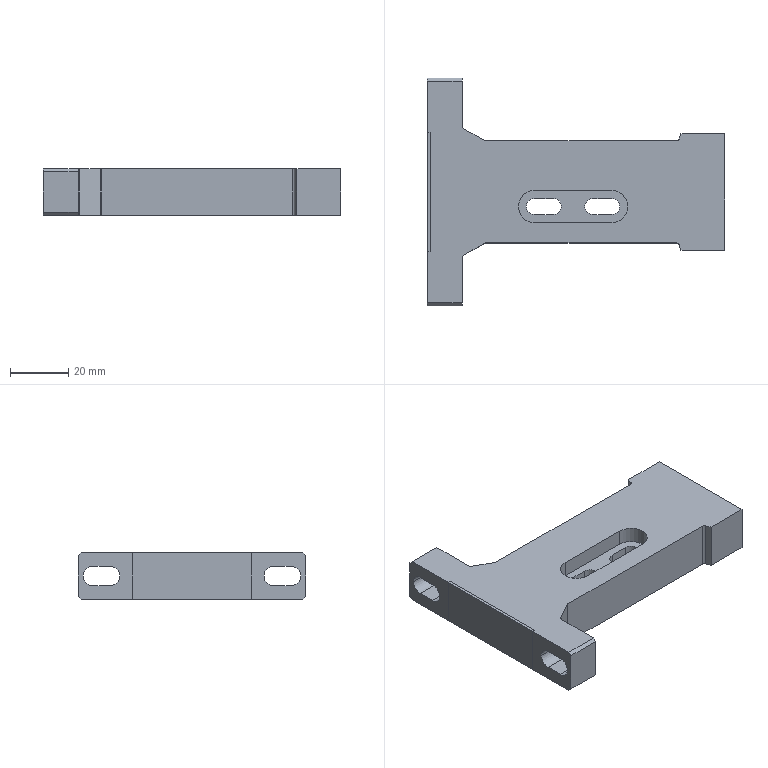NC program | NX | posted with a generic post | part box 102 x 78 x 16 mm
Lines 23 to 1003 of 11044:
(ADAPTIVE_MILLING , TOOL : D10)
N44 T10 M6
N46 G54
N48 G17 G0 G90 X-61.696 Y-0.049 B0. C0. S9500 M3
N50 G43 Z30. H10
N52 Z-15.
N54 G94 G1 Z-16. F1000.
N56 X-60.339 Y-0.579 F3000.
N58 G3 X-59.049 Y-0.049 R1.015
N60 X-58.405 Y3.11 R9.424
N62 X-58.209 Y14.606 R185.073
N64 G1 X-58.207 Y20.006
N66 Y39.206
N68 X-58.205 Y39.406
N70 X-58.201 Y39.506
N72 X-58.195 Y39.606
N74 X-58.186 Y39.706
N76 G2 X-55.275 Y44.039 R6.033
N78 X-49.705 Y45.827 R13.143
N80 X-41.117 Y46.175 R79.783
N82 G1 X-39.617 Y46.182
N84 X-37.517 Y46.186
N86 X-33.917 Y46.189
N88 X-19.717 Y46.19
N90 X51.283
N92 X51.383 Y46.189
N94 G2 X55.859 Y43.528 R5.822
N96 X57.771 Y38.109 R12.333
N98 X58.168 Y30.025 R65.613
N100 G1 X58.175 Y28.925
N102 X58.182 Y27.425
N104 X58.186 Y25.225
N106 X58.189 Y21.325
N108 X58.19 Y0.425
N110 Y-39.275
N112 G2 X55.694 Y-43.737 R5.724
N114 X50.313 Y-45.74 R11.882
N116 X42.231 Y-46.167 R61.694
N118 G1 X41.131 Y-46.175
N120 X39.631 Y-46.182
N122 X37.531 Y-46.186
N124 X33.931 Y-46.189
N126 X20.031 Y-46.19
N128 X-51.269
N130 G2 X-55.733 Y-43.7 R5.711
N132 X-57.755 Y-38.222 R11.964
N134 X-58.168 Y-30.038 R63.41
N136 G1 X-58.176 Y-28.938
N138 X-58.182 Y-27.338
N140 X-58.187 Y-25.038
N142 X-58.189 Y-20.838
N144 X-58.19 Y-3.438
N146 X-58.188 Y-3.238
N148 G2 X-57.69 Y2.539 R147.004
N150 G3 X-57.421 Y15.233 R195.936
N152 G1 X-57.417 Y18.533
N154 X-57.416 Y26.333
N156 Y36.533
N158 X-57.412 Y36.733
N160 X-57.404 Y36.933
N162 X-57.398 Y37.033
N164 G2 X-55.508 Y41.459 R7.653
N166 X-52.31 Y43.982 R5.373
N168 X-44.94 Y45.217 R25.854
N170 X-29.642 Y45.381 R372.439
N172 G1 X-12.542 Y45.382
N174 X48.458
N176 X48.658 Y45.38
N178 X48.858 Y45.374
N180 X48.958 Y45.37
N182 X49.058 Y45.364
N184 G2 X55.038 Y41.512 R7.654
N186 X56.975 Y35.255 R15.486
N188 X57.368 Y24.969 R95.347
N190 G1 X57.374 Y23.169
N192 X57.378 Y20.669
N194 X57.381 Y15.869
N196 Y-36.531
N198 Y-36.631
N200 X57.376 Y-36.831
N202 G2 X53.616 Y-42.969 R7.597
N204 X47.477 Y-44.947 R15.163
N206 X38.492 Y-45.359 R77.926
N208 G1 X37.092 Y-45.368
N210 X35.192 Y-45.374
N212 X32.692 Y-45.379
N214 X28.092 Y-45.381
N216 X-48.508 Y-45.382
N218 X-48.708 Y-45.38
N220 G2 X-53.361 Y-43.555 R7.348
N222 X-55.982 Y-40.31 R5.331
N224 X-57.199 Y-33.239 R25.363
N226 X-57.38 Y-19.342 R303.882
N228 X-57.337 Y-3.642 R758.305
N230 G3 X-56.702 Y7.738 R243.944
N232 X-56.625 Y23.138 R782.696
N234 G2 X-56.584 Y35.137 R471.558
N236 X-56.15 Y37.43 R14.71
N238 X-55.948 Y40.397 R12.45
N240 G1 X-55.489 Y41.505
N242 G2 X-53.511 Y43.486 R5.689
N244 X-50.966 Y44.15 R6.048
N246 G3 X-44.072 Y44.433 R195.122
N248 G2 X-26.374 Y44.572 R665.674
N250 G1 X-1.874 Y44.573
N252 X24.926
N254 X25.926 Y44.577
N256 X27.526 Y44.579
N258 X28.926 Y44.578
N260 X29.726 Y44.58
N262 G2 X47.125 Y44.547 R975.438
N264 X54.234 Y39.846 R8.79
N266 X56.184 Y32.965 R18.1
N268 X56.559 Y22.176 R112.451
N270 G1 X56.565 Y20.276
N272 X56.57 Y17.476
N274 X56.572 Y12.276
N276 Y-34.224
N278 X56.57 Y-34.424
N280 X56.565 Y-34.624
N282 G2 X51.84 Y-42.232 R8.781
N284 X45.159 Y-44.162 R17.772
N286 X35.472 Y-44.553 R97.042
N288 G1 X33.972 Y-44.56
N290 X32.072 Y-44.566
N292 X29.172 Y-44.57
N294 X23.572 Y-44.573
N296 X-46.228
N298 X-46.428 Y-44.57
N300 G2 X-49.297 Y-44.15 R11.706
N302 X-52.397 Y-43.948 R13.168
N304 G1 X-53.413 Y-43.527
N306 G3 X-54. Y-43.472 R1.048
N308 G1 X-54.744 Y-43.627
N310 X-56.702 Y-44.036 Z-15.9
N312 G2 X-57.913 Y-43.527 R1.026
N314 G1 X-58.683 Y-41.959
N316 G2 X-59.435 Y-39.463 R12.103
N318 X-59.96 Y-35.767 R25.244
N320 X-60.33 Y-26.409 R134.501
N322 G1 X-60.397 Y23.087
N324 G2 X-59.526 Y36.542 R103.005
N326 G1 X-58.808 Y42.001
N328 G2 X-57.761 Y44.124 R3.712
N330 X-55.824 Y45.682 R11.903
N332 G1 X-53.248 Y47.332
N334 G2 X-51.773 Y46.843 R1.003
N336 G1 X-51.686 Y46.614
N338 X-50.979 Y44.743 Z-16.
N340 G3 X-50.066 Y44.15 R1.01
N342 G1 X-39.034
N344 X-38.966 Y44.146
N346 G3 X-31.78 Y43.799 R53.744
N348 G1 X-30.48 Y43.791
N350 X-28.68 Y43.786
N352 X-25.78 Y43.783
N354 X-17.08 Y43.782
N356 X-12.18 Y43.781
N358 X-11.18 Y43.778
N360 X-9.58 Y43.776
N362 X-8.18 Y43.777
N364 X-7.48 Y43.775
N366 X-6.28 Y43.776
N368 X-5.38 Y43.774
N370 X-4.38 Y43.775
N372 X-3.58 Y43.773
N374 X-2.58 Y43.775
N376 X-1.48 Y43.772
N378 X-0.48 Y43.774
N380 X0.42 Y43.773
N382 X1.52 Y43.774
N384 X2.52 Y43.772
N386 X3.52 Y43.774
N388 X4.42 Y43.773
N390 X5.52 Y43.775
N392 X6.52 Y43.774
N394 X8.02 Y43.775
N396 X9.02 Y43.773
N398 X10.02 Y43.774
N400 X11.12 Y43.772
N402 X12.32 Y43.775
N404 X13.32 Y43.772
N406 X14.22 Y43.774
N408 X15.52 Y43.772
N410 X16.32 Y43.773
N412 X17.32 Y43.772
N414 X18.12 Y43.773
N416 X19.12 Y43.772
N418 X20.22 Y43.774
N420 X21.12 Y43.772
N422 X22.22 Y43.774
N424 X22.92 Y43.773
N426 X24.02 Y43.776
N428 X24.92 Y43.775
N430 X25.72 Y43.777
N432 X26.62
N434 X27.62 Y43.779
N436 X28.72 Y43.778
N438 X29.62 Y43.779
N440 X30.72 Y43.778
N442 X31.92 Y43.781
N444 X33.02 Y43.779
N446 X34.02 Y43.781
N448 X35.02 Y43.78
N450 X36.02 Y43.782
N452 X37.22 Y43.78
N454 X38.12 Y43.782
N456 X39.22 Y43.78
N458 G2 X45.717 Y43.708 R100.202
N460 X53.427 Y38.364 R9.62
N462 X55.369 Y31.168 R19.833
N464 X55.745 Y21.979 R108.354
N466 X56.15 Y19.966 R6.877
N468 G1 Y-19.966
N470 X56.146 Y-20.034
N472 G3 X55.804 Y-27.02 R54.496
N474 G2 X55.707 Y-33.718 R116.335
N476 X50.273 Y-41.475 R9.663
N478 X43.264 Y-43.357 R19.765
N480 X32.075 Y-43.749 R117.383
N482 G1 X30.175 Y-43.756
N484 X27.575 Y-43.761
N486 X23.175 Y-43.763
N488 X6.575 Y-43.764
N490 X-32.425 Y-43.765
N492 X-33.425 Y-43.768
N494 G3 X-37.222 Y-43.802 R98.297
N496 G2 X-39.034 Y-44.15 R6.039
N498 G1 X-49.334
N500 G3 X-50.286 Y-44.824 R1.032
N502 G1 X-51.14 Y-46.633 Z-15.9
N504 G2 X-51.555 Y-47.217 R1.332
N506 X-52.516 Y-47.332 R1.014
N508 G1 X-53.837 Y-46.797
N510 X-55.151 Y-46.246
N512 G2 X-57.112 Y-44.577 R5.529
N514 X-59.082 Y-40.59 R10.831
N516 X-59.861 Y-36.309 R26.439
N518 X-60.306 Y-28.834 R85.26
N520 G1 X-60.811 Y11.791
N522 G2 X-59.964 Y31.743 R183.166
N524 G1 X-59.113 Y40.451
N526 G2 X-57.814 Y43.873 R6.784
N528 G1 X-57.411 Y44.339
N530 X-56.967 Y44.765
N532 X-55.695 Y45.831
N534 G2 X-53.383 Y46.858 R6.114
N536 X-51.413 Y47.094 R9.628
N538 G1 X-41.256 Y47.21
N540 G2 X-40.35 Y46.678 R1.059
N542 G1 X-39.19 Y45.048 Z-16.
N544 X-38.928 Y44.676
N546 X-38.652 Y44.314
N548 G3 X-38.074 Y44.028 R1.041
N550 G2 X-36.759 Y43.638 R6.047
N552 G3 X-31.501 Y43.076 R24.558
N554 X-10.701 Y42.984 R997.948
N556 G1 X-9.801 Y42.98
N558 X-8.801
N560 X-7.801 Y42.977
N562 X-6.701
N564 X-5.801 Y42.975
N566 X-4.701 Y42.976
N568 X-3.801 Y42.974
N570 X-2.701 Y42.975
N572 X-1.701 Y42.973
N574 X-0.601 Y42.975
N576 X0.299 Y42.973
N578 X1.399 Y42.974
N580 X2.599 Y42.973
N582 X3.499 Y42.974
N584 X4.499 Y42.973
N586 X5.399 Y42.974
N588 X6.499 Y42.973
N590 X7.399 Y42.974
N592 X8.099 Y42.973
N594 X8.699 Y42.972
N596 X9.899 Y42.974
N598 X10.799 Y42.973
N600 X11.999 Y42.974
N602 X13.099 Y42.972
N604 X13.899 Y42.973
N606 X14.999 Y42.972
N608 X15.899 Y42.973
N610 X16.899 Y42.972
N612 X17.899 Y42.973
N614 X18.899 Y42.972
N616 X19.999 Y42.974
N618 X20.799 Y42.973
N620 X21.899 Y42.974
N622 X22.799
N624 X23.799 Y42.976
N626 X24.599 Y42.975
N628 X25.599 Y42.977
N630 X26.599 Y42.976
N632 X27.599 Y42.979
N634 X28.499 Y42.977
N636 X29.499 Y42.979
N638 X30.599 Y42.978
N640 X31.599 Y42.98
N642 X32.499 Y42.979
N644 X33.499 Y42.98
N646 X34.699 Y42.979
N648 X35.699 Y42.98
N650 X36.899 Y42.979
N652 X37.799 Y42.981
N654 X38.699 Y42.98
N656 G2 X44.494 Y42.862 R60.009
N658 X52.545 Y37.151 R10.26
N660 X54.542 Y29.658 R20.907
N662 X54.921 Y23.471 R166.403
N664 G3 X55.486 Y22.511 R3.073
N666 G1 X55.793 Y21.772
N668 G3 X57.395 Y21.42 R1.002
N670 X57.73 Y22.257 Z-15.954 R1.157
N672 G1 X57.829 Y23.325 Z-15.9
N674 X58.043 Y25.669
N676 X58.044 Y26.793
N678 X58.003 Y27.915
N680 X57.918 Y28.658
N682 X57.797 Y29.395
N684 X57.299 Y31.907
N686 X56.779 Y34.416
N688 G3 X54.442 Y40.023 R18.405
N690 X53.13 Y41.838 R17.042
N692 X51.059 Y43.614 R10.805
N694 X48.171 Y45.047 R11.002
N696 X44.023 Y45.813 R18.815
N698 G1 X40.589 Y45.906
N700 X37.155 Y45.977
N702 X31.742 Y46.089
N704 X26.328 Y46.184
N706 X20.914 Y46.263
N708 X-34.052 Y46.977
N710 X-34.268 Y46.952
N712 X-34.477 Y46.889
N714 X-36.225 Y46.099
N716 X-36.824 Y45.834 Z-15.933
N718 X-37.413 Y45.546 Z-15.966
N720 G3 X-37.811 Y45. Z-16. R1.038
N722 X-37.234 Y43.795 R1.005
N724 X-35.065 Y42.922 R18.806
N726 X-29.01 Y42.29 R29.09
N728 X-9.111 Y42.182 R961.396
N730 G1 X-8.211 Y42.179
N732 X-7.111
N734 X-6.011 Y42.176
N736 X-5.111 Y42.177
N738 X-4.111 Y42.175
N740 X-2.911 Y42.176
N742 X-2.111 Y42.175
N744 X-1.011 Y42.176
N746 X-0.111 Y42.174
N748 X0.989 Y42.175
N750 X2.089 Y42.173
N752 X3.089 Y42.175
N754 X3.989 Y42.173
N756 X4.989 Y42.175
N758 X5.989 Y42.173
N760 X6.589 Y42.174
N762 X7.189 Y42.175
N764 X8.289 Y42.173
N766 X9.489 Y42.175
N768 X10.489 Y42.173
N770 X11.589 Y42.174
N772 X12.489 Y42.173
N774 X13.389 Y42.174
N776 X14.489 Y42.172
N778 X15.389 Y42.173
N780 X16.589 Y42.171
N782 X17.589 Y42.173
N784 X18.489 Y42.172
N786 X19.589 Y42.174
N788 X20.589 Y42.173
N790 X21.589 Y42.175
N792 X22.389 Y42.174
N794 X23.489 Y42.177
N796 X24.289 Y42.176
N798 G2 X41.889 Y42.144 R960.225
N800 X51.822 Y35.711 R10.952
N802 X53.738 Y28.089 R22.597
N804 G3 X54.139 Y24.313 R37.745
N806 X54.684 Y23.587 R1.564
N808 G1 X55.11 Y23.032
N810 G3 X56.394 Y22.769 R1.005
N812 X56.906 Y23.587 Z-15.95 R1.037
N814 G1 X57.058 Y24.57 Z-15.9
N816 X57.378 Y26.697
N818 X57.36 Y26.929
N820 X56.45 Y31.419
N822 G3 X54.559 Y37.132 R31.395
N824 X51.753 Y41.204 R14.283
N826 X49.547 Y43.019 R16.552
N828 X46.484 Y44.351 R11.212
N830 X42.194 Y45.053 R20.306
N832 G1 X41.573 Y45.069
N834 X-32.473 Y45.668
N836 X-33.631 Y45.524
N838 X-34.786 Y45.357
N840 X-36.042 Y45.171 Z-15.964
N842 G3 X-36.611 Y44.74 Z-16. R1.031
N844 X-36.37 Y43.418 R1.005
N846 X-33.098 Y42.028 R6.676
N848 X-25.427 Y41.465 R47.463
N850 X-7.428 Y41.38 R986.405
N852 G1 X-6.528 Y41.377
N854 X-5.428 Y41.378
N856 X-4.528 Y41.377
N858 X-3.428
N860 X-2.328 Y41.375
N862 X-1.528 Y41.376
N864 X-0.428 Y41.374
N866 X0.672 Y41.375
N868 X1.672 Y41.374
N870 X2.672 Y41.375
N872 X3.772 Y41.373
N874 X4.872 Y41.375
N876 X5.872 Y41.373
N878 X6.972 Y41.375
N880 X7.972 Y41.374
N882 X8.972 Y41.375
N884 X9.972 Y41.373
N886 X11.072 Y41.375
N888 X12.072 Y41.373
N890 X13.172 Y41.374
N892 X14.072 Y41.373
N894 X15.172 Y41.374
N896 X15.872 Y41.373
N898 X16.372 Y41.372
N900 X17.272 Y41.374
N902 X18.372 Y41.373
N904 X19.372 Y41.374
N906 X20.272 Y41.373
N908 X21.172 Y41.375
N910 X22.172 Y41.374
N912 X23.072 Y41.376
N914 X24.072 Y41.375
N916 G2 X40.572 Y41.332 R857.039
N918 X48.013 Y38.575 R11.667
N920 X52.019 Y31.778 R13.914
N922 X53.068 Y26.079 R48.797
N924 G3 X53.594 Y24.477 R3.965
N926 G1 X53.661 Y24.403
N928 X53.704 Y24.361
N930 X54.498 Y23.752
N932 G3 X55.572 Y23.661 R1.011
N934 X56.1 Y24.394 Z-15.953 R1.047
N936 G1 X56.36 Y25.426 Z-15.9
N938 X56.59 Y26.317
N940 X56.801 Y27.213
N942 X56.795 Y27.434
N944 X56.748 Y27.649
N946 X54.228 Y34.706
N948 G3 X51.757 Y39.01 R14.738
N950 G1 X50.642 Y40.355
N952 G3 X47.443 Y42.683 R10.498
N954 X44.915 Y43.673 R17.158
N956 X42.21 Y44.125 R14.036
N958 X37.227 Y44.4 R62.062
N960 G1 X-31.997 Y45.303
N962 X-32.148 Y45.293
N964 X-34.302 Y44.993
N966 X-34.949 Y44.908 Z-15.933
N968 X-35.593 Y44.798 Z-15.965
N970 G3 X-36.13 Y44.381 Z-16. R1.038
N972 X-35.894 Y43.053 R1.005
N974 X-32.324 Y41.357 R7.062
N976 X-24.863 Y40.702 R42.27
N978 X-3.764 Y40.578 R958.475
N980 G1 X-2.664 Y40.575
N982 X-1.564 Y40.577
N984 X-0.664 Y40.575
N986 X0.436 Y40.576
N988 X1.536 Y40.574
N990 X2.636 Y40.575
N992 X3.636 Y40.574
N994 X4.636 Y40.575
N996 X5.636 Y40.573
N998 X6.736 Y40.575
N1000 X7.736 Y40.573
N1002 X8.736 Y40.575
N1004 X9.836 Y40.573
N1006 X10.836 Y40.574
N1008 X11.836 Y40.573
N1010 X12.936 Y40.574
N1012 X13.936 Y40.572
N1014 X14.936 Y40.574
N1016 X16.036 Y40.572
N1018 X17.036 Y40.574
N1020 X17.936 Y40.573
N1022 X19.136 Y40.575
N1024 X19.936 Y40.574
N1026 X20.936 Y40.575
N1028 X21.936
N1030 X23.036 Y40.577
N1032 X23.936 Y40.575
N1034 X25.036 Y40.577
N1036 X25.936
N1038 X27.036 Y40.579
N1040 X27.936 Y40.578
N1042 X29.136 Y40.58
N1044 G2 X39.635 Y40.501 R270.355
N1046 X47.564 Y37.182 R11.847
N1048 X51.277 Y30.313 R15.008
N1050 G3 X52.373 Y25.847 R98.559
N1052 X53.175 Y24.626 R1.996
N1054 G1 X53.709 Y24.357
N1056 G3 X55.021 Y24.439 R1.005
N1058 X55.298 Y25.373 Z-15.949 R1.036
N1060 G1 X55.175 Y26.351 Z-15.9
N1062 X54.874 Y28.704
N1064 X54.224 Y31.245
N1066 G3 X53.178 Y34.044 R20.782
N1068 G1 X52.152 Y36.238
N1070 G3 X49.467 Y39.667 R11.906
N1072 X45.885 Y42.11 R14.093
N1074 X41.601 Y43.288 R13.936
N1076 X38.622 Y43.507 R29.824
N1078 G1 X-31.611 Y44.931
N1080 X-33.752 Y44.569
N1082 X-34.399 Y44.463 Z-15.933
N1084 X-35.041 Y44.333 Z-15.966
N1086 G3 X-35.564 Y43.905 Z-16. R1.038
N1088 X-35.413 Y42.683 R1.007
N1090 X-32.83 Y41.002 R4.908
N1092 X-26.322 Y40.024 R26.023
N1094 X-8.025 Y39.787 R468.491
N1096 G1 X-7.225 Y39.784
N1098 X-6.125 Y39.783
N1100 X-5.225 Y39.78
N1102 X-4.025
N1104 X-3.025 Y39.777
N1106 X-1.825 Y39.778
N1108 X-0.825 Y39.775
N1110 X0.275 Y39.776
N1112 X1.275 Y39.774
N1114 X2.375 Y39.776
N1116 X3.375 Y39.774
N1118 X4.475 Y39.775
N1120 X5.275 Y39.774
N1122 X6.375 Y39.775
N1124 X7.275 Y39.774
N1126 X8.375 Y39.775
N1128 X9.375 Y39.773
N1130 X10.275 Y39.774
N1132 X11.375 Y39.773
N1134 X12.375 Y39.774
N1136 X13.375 Y39.772
N1138 X14.575 Y39.774
N1140 X15.475 Y39.773
N1142 X16.575 Y39.775
N1144 X17.275 Y39.774
N1146 X17.875 Y39.773
N1148 X18.775 Y39.775
N1150 X19.775 Y39.774
N1152 X20.675 Y39.775
N1154 X21.675 Y39.774
N1156 X22.575 Y39.776
N1158 X23.675 Y39.775
N1160 G2 X37.974 Y39.717 R566.887
N1162 X44.892 Y37.696 R13.295
N1164 X49.861 Y31.095 R13.415
N1166 G1 X49.931 Y30.908
N1168 X50. Y30.72
N1170 X50.1 Y30.438
N1172 X50.198 Y30.154
N1174 X50.324 Y29.774
N1176 X50.416 Y29.489
N1178 X50.565 Y29.011
N1180 X50.827 Y28.15
N1182 X50.945 Y27.768
N1184 X51.006 Y27.578
N1186 X51.131 Y27.198
N1188 X51.229 Y26.914
N1190 X51.297 Y26.726
N1192 X51.368 Y26.539
N1194 X51.405 Y26.446
N1196 G3 X52.285 Y25.016 R3.226
N1198 G1 X52.37 Y24.963
N1200 X52.4 Y24.947
N1202 X53.232 Y24.602
N1204 G3 X54.316 Y24.814 R1.01
N1206 X54.61 Y25.661 Z-15.954 R1.048
N1208 G1 X54.57 Y26.732 Z-15.9
N1210 X54.536 Y27.707
N1212 X54.486 Y28.68
N1214 X54.397 Y28.949
N1216 X52.974 Y31.8
N1218 X51.536 Y34.644
N1220 G3 X49.286 Y38.084 R26.114
N1222 X47.355 Y39.822 R8.912
N1224 X43.472 Y41.776 R18.103
N1226 X40.198 Y42.498 R16.752
N1228 G1 X39.081 Y42.609
N1230 X37.961 Y42.672
N1232 X-31.353 Y44.595
N1234 X-33.382 Y44.179
N1236 X-34.043 Y44.046 Z-15.934
N1238 X-34.7 Y43.891 Z-15.968
N1240 G3 X-35.191 Y43.483 Z-16. R1.042
N1242 X-35.134 Y42.349 R1.01
N1244 X-32.337 Y40.362 R5.089
N1246 X-25.746 Y39.275 R25.077
N1248 X-9.65 Y38.996 R345.711
N1250 G1 X-8.75 Y38.993
N1252 X-8.15 Y38.992
N1254 X-7.25 Y38.988
N1256 X-6.45 Y38.986
N1258 X-5.95
N1260 X-5.05 Y38.982
N1262 X-4.05
N1264 X-3.25 Y38.979
N1266 X-2.15 Y38.98
N1268 X-1.25 Y38.977
N1270 X-0.15 Y38.978
N1272 X0.95 Y38.975
N1274 X1.95 Y38.976
N1276 X2.95 Y38.974
N1278 X3.85 Y38.975
N1280 X4.95 Y38.974
N1282 X6.05 Y38.976
N1284 X6.95 Y38.974
N1286 X8.25 Y38.975
N1288 X9.15 Y38.973
N1290 X10.15 Y38.975
N1292 X11.05 Y38.973
N1294 X12.15 Y38.975
N1296 X13.25 Y38.973
N1298 X14.05 Y38.974
N1300 X15.25 Y38.972
N1302 X16.25 Y38.974
N1304 X17.15 Y38.973
N1306 X18.25 Y38.975
N1308 X19.15 Y38.974
N1310 X20.25 Y38.976
N1312 X21.35 Y38.974
N1314 X22.15 Y38.976
N1316 X23.25 Y38.975
N1318 X24.35 Y38.978
N1320 X25.35 Y38.976
N1322 X26.45 Y38.979
N1324 G2 X37.148 Y38.888 R257.583
N1326 X44.361 Y36.527 R13.227
N1328 X48.849 Y30.629 R14.128
N1330 G3 X50.649 Y26.397 R96.462
N1332 X51.709 Y25.103 R2.823
N1334 G1 X51.802 Y25.066
N1336 X51.898 Y25.036
N1338 X51.934 Y25.027
N1340 X52.265 Y24.984
N1342 X52.397 Y24.948
N1344 X52.489 Y24.91
N1346 G3 X53.567 Y25.115 R1.01
N1348 X53.869 Y25.954 Z-15.954 R1.049
N1350 G1 X53.845 Y27.032 Z-15.9
N1352 X53.795 Y28.88
N1354 X53.74 Y29.074
N1356 X53.654 Y29.257
N1358 X51.858 Y32.113
N1360 X50.044 Y34.959
N1362 G3 X46.657 Y38.574 R15.762
N1364 G1 X45.896 Y39.108
N1366 X45.104 Y39.595
N1368 X44.016 Y40.205
N1370 X42.916 Y40.795
N1372 G3 X41.744 Y41.191 R4.606
N1374 X38.295 Y41.723 R33.782
N1376 G1 X36.802 Y41.804
N1378 X19.934 Y42.163
N1380 X12.436 Y42.301
N1382 X-30.474 Y42.966
N1384 X-32.658 Y43.248
N1386 X-33.307 Y43.338 Z-15.933
N1388 X-33.958 Y43.401 Z-15.966
N1390 G3 X-34.584 Y43.145 Z-16. R1.038
N1392 X-34.708 Y41.794 R1.005
N1394 X-32.295 Y39.875 R4.653
N1396 X-26.349 Y38.62 R20.613
N1398 X-13.958 Y38.231 R167.808
N1400 G1 X-12.558 Y38.217
N1402 X-11.158 Y38.207
N1404 X-9.758 Y38.2
N1406 X-8.158 Y38.196
N1408 X-7.358 Y38.192
N1410 X-6.458 Y38.19
N1412 X-5.858 Y38.188
N1414 X-5.158 Y38.185
N1416 X-4.058 Y38.184
N1418 X-3.158 Y38.181
N1420 X-2.158
N1422 X-1.258 Y38.179
N1424 X-0.058
N1426 X0.842 Y38.177
N1428 X1.642
N1430 X2.742 Y38.175
N1432 X3.742 Y38.176
N1434 X4.542 Y38.175
N1436 X5.542 Y38.176
N1438 X6.542 Y38.174
N1440 X7.642 Y38.176
N1442 X8.642 Y38.174
N1444 X9.542 Y38.175
N1446 X10.642 Y38.173
N1448 X11.542 Y38.174
N1450 X12.742 Y38.172
N1452 X13.742 Y38.174
N1454 X14.742 Y38.173
N1456 X15.742 Y38.174
N1458 X16.642 Y38.173
N1460 X17.542 Y38.175
N1462 X18.642 Y38.174
N1464 X19.742 Y38.176
N1466 X20.642 Y38.174
N1468 G2 X35.541 Y38.105 R546.78
N1470 X42.437 Y36.308 R14.625
N1472 X47.727 Y30.45 R14.256
N1474 G3 X49.868 Y26.38 R65.983
N1476 X51.033 Y25.175 R3.038
N1478 G1 X51.128 Y25.143
N1480 X51.212 Y25.122
N1482 X52.005 Y25.018
N1484 G3 X53.002 Y25.51 R1.01
N1486 X53.055 Y26.413 Z-15.953 R1.047
N1488 G1 X52.724 Y27.424 Z-15.9
N1490 X52.064 Y29.41
N1492 X50.674 Y31.634
N1494 X49.261 Y33.844
N1496 G3 X46.266 Y37.339 R22.005
N1498 X42.912 Y39.463 R12.847
N1500 X38.148 Y40.788 R14.229
N1502 X33.177 Y41.166 R49.65
N1504 G1 X-30.208 Y42.678
N1506 X-32.368 Y42.817
N1508 X-33.03 Y42.865 Z-15.933
N1510 X-33.693 Y42.889 Z-15.966
N1512 G3 X-34.29 Y42.608 Z-16. R1.04
N1514 X-34.514 Y41.511 R1.01
N1516 X-32.684 Y39.61 R3.668
N1518 X-27.434 Y38.071 R15.447
N1520 X-17.957 Y37.502 R81.354
N1522 X4.242 Y37.376 R991.029
N1524 G1 X5.142
N1526 X6.142 Y37.375
N1528 X7.142 Y37.376
N1530 X8.042 Y37.374
N1532 X9.142 Y37.375
N1534 X10.042 Y37.373
N1536 X11.242 Y37.375
N1538 X12.342 Y37.373
N1540 X13.142 Y37.374
N1542 X14.242 Y37.373
N1544 X15.242 Y37.375
N1546 X16.342 Y37.373
N1548 X17.242 Y37.374
N1550 X18.542 Y37.373
N1552 X19.542 Y37.376
N1554 G2 X34.341 Y37.301 R558.568
N1556 X41.267 Y35.592 R15.442
N1558 X46.586 Y30.281 R14.932
N1560 G3 X49.09 Y26.306 R62.467
N1562 X50.347 Y25.195 R3.107
N1564 G1 X51.232 Y25.119
N1566 G3 X52.231 Y25.614 R1.01
N1568 X52.286 Y26.509 Z-15.954 R1.048
N1570 G1 X51.959 Y27.531 Z-15.9
N1572 X51.385 Y29.324
N1574 X51.317 Y29.476
N1576 X51.232 Y29.619
N1578 X49.861 Y31.453
N1580 X48.472 Y33.274
N1582 G3 X45.584 Y36.246 R23.367
N1584 G1 X44.248 Y37.375
N1586 G3 X41.424 Y38.913 R10.884
N1588 X35.341 Y40.153 R22.514
N1590 G1 X32.851 Y40.323
N1592 X30.357 Y40.439
N1594 X-30.084 Y42.4
N1596 X-32.232 Y42.539
N1598 X-32.902 Y42.587 Z-15.934
N1600 X-33.574 Y42.612 Z-15.967
N1602 G3 X-34.16 Y42.346 Z-16. R1.041
N1604 X-34.399 Y41.234 R1.01
N1606 X-32.38 Y38.985 R3.994
N1608 X-26.758 Y37.308 R16.141
N1610 X-16.583 Y36.703 R86.673
N1612 X5.816 Y36.576 R992.042
N1614 G1 X6.816
N1616 X7.816 Y36.574
N1618 X8.816 Y36.575
N1620 X9.916 Y36.574
N1622 X11.016 Y36.575
N1624 X12.016 Y36.573
N1626 X13.016 Y36.575
N1628 X14.016 Y36.573
N1630 X15.216 Y36.575
N1632 X16.016 Y36.574
N1634 X17.216 Y36.575
N1636 X18.116 Y36.574
N1638 X19.116 Y36.576
N1640 X20.016 Y36.575
N1642 X21.216 Y36.577
N1644 X22.216 Y36.576
N1646 G2 X33.715 Y36.468 R263.238
N1648 X41.365 Y34.134 R14.892
N1650 X45.984 Y29.335 R18.116
N1652 G3 X48.722 Y25.772 R25.252
N1654 X49.807 Y25.15 R1.934
N1656 G1 X50.607
N1658 G3 X51.49 Y25.682 R1.011
N1660 X51.528 Y26.584 Z-15.954 R1.155
N1662 G1 X51.266 Y27.621 Z-15.9
N1664 X50.827 Y29.316
N1666 X50.73 Y29.492
N1668 X50.607 Y29.65
N1670 X47.96 Y32.305
N1672 X45.297 Y34.943
N1674 G3 X37.669 Y38.943 R16.808
N1676 G1 X36.751 Y39.106
N1678 X35.826 Y39.215
N1680 G3 X28.349 Y39.687 R156.578
N1682 G1 X-29.85 Y41.846
N1684 X-31.998 Y41.984
N1686 X-32.67 Y42.032 Z-15.934
N1688 X-33.344 Y42.058 Z-15.967
N1690 G3 X-33.927 Y41.794 Z-16. R1.042
N1692 X-34.169 Y40.68 R1.01
N1694 X-32.177 Y38.397 R4.045
N1696 X-26.588 Y36.616 R15.873
N1698 X-16.419 Y35.926 R78.512
N1700 X6.48 Y35.777 R964.551
N1702 G1 X7.48 Y35.775
N1704 X8.58 Y35.776
N1706 X9.58 Y35.774
N1708 X10.68 Y35.775
N1710 X11.78 Y35.773
N1712 X12.78 Y35.775
N1714 X13.88 Y35.773
N1716 X14.88 Y35.775
N1718 X15.88 Y35.774
N1720 X16.98 Y35.776
N1722 X17.88 Y35.774
N1724 X18.98 Y35.776
N1726 X20.18 Y35.775
N1728 X21.18 Y35.777
N1730 X22.28 Y35.776
N1732 X23.18
N1734 G2 X33.077 Y35.632 R170.726
N1736 X43.955 Y30.235 R15.012
N1738 G3 X47.237 Y26.333 R213.925
N1740 X48.729 Y25.185 R4.192
N1742 X49.826 Y25.15 R13.591
N1744 X50.79 Y25.885 R1.007
N1746 X50.531 Y26.883 Z-15.946 R1.11
N1748 G1 X49.993 Y27.635 Z-15.9
N1750 X48.962 Y29.073
N1752 X47.968 Y30.537
N1754 G3 X46.354 Y32.423 R10.707
N1756 G1 X44.414 Y34.188
N1758 G3 X40.383 Y36.89 R22.663
N1760 X36.853 Y38.062 R11.87
N1762 X30.659 Y38.754 R52.808
N1764 G1 X-29.724 Y41.562
N1766 X-31.834 Y41.621
N1768 X-32.523 Y41.644 Z-15.935
N1770 X-33.213 Y41.647 Z-15.969
N1772 G3 X-33.766 Y41.389 Z-16. R1.045
N1774 X-34.052 Y40.397 R1.011
N1776 X-32.725 Y38.314 R3.194
N1778 X-27.805 Y36.199 R12.215
N1780 X-18.77 Y35.231 R50.619
N1782 X8.428 Y34.976 R883.859
N1784 G1 X9.528 Y34.975
N1786 X10.628 Y34.976
N1788 X11.628 Y34.974
N1790 X12.728 Y34.976
N1792 X13.828 Y34.974
N1794 X14.728 Y34.975
N1796 X15.728 Y34.974
N1798 X16.928 Y34.976
N1800 X17.828 Y34.975
N1802 X18.928 Y34.976
N1804 X19.928 Y34.975
N1806 X20.828 Y34.976
N1808 X22.028 Y34.974
N1810 X23.028 Y34.975
N1812 X24.128 Y34.973
N1814 X25.028 Y34.974
N1816 X25.828 Y34.971
N1818 G2 X33.318 Y34.693 R65.382
N1820 X42.922 Y29.801 R15.837
N1822 G3 X46.519 Y26.048 R136.303
N1824 X47.839 Y25.171 R3.572
N1826 G1 X47.938 Y25.154
N1828 X47.975 Y25.15
N1830 X48.975
N1832 G3 X49.938 Y25.882 R1.007
N1834 X49.683 Y26.88 Z-15.946 R1.11
N1836 G1 X49.148 Y27.635 Z-15.9
N1838 X47.919 Y29.368
N1840 X47.81 Y29.497
N1842 X45.063 Y32.227
N1844 G3 X40.204 Y35.683 R21.298
N1846 X32.311 Y37.726 R19.064
N1848 G1 X-29.49 Y40.066
N1850 X-29.786 Y40.123
N1852 X-31.555 Y40.748
N1854 X-32.186 Y40.975 Z-15.934
N1856 X-32.825 Y41.182 Z-15.967
N1858 G3 X-33.463 Y41.083 Z-16. R1.041
N1860 X-33.99 Y40.066 R1.01
N1862 X-32.669 Y37.8 R3.253
N1864 X-27.903 Y35.585 R11.903
N1866 X-19.086 Y34.491 R45.145
N1868 X4.51 Y34.182 R617.529
N1870 G1 X5.31 Y34.179
N1872 X6.41
N1874 X7.31 Y34.177
N1876 X8.41 Y34.178
N1878 X9.31 Y34.176
N1880 X10.41
N1882 X11.41 Y34.175
N1884 X12.51 Y34.176
N1886 X13.51 Y34.174
N1888 X14.51 Y34.175
N1890 X15.61 Y34.174
N1892 X16.71 Y34.176
N1894 X17.71 Y34.175
N1896 X18.71 Y34.176
N1898 X19.81 Y34.174
N1900 G2 X30.907 Y34.026 R192.564
N1902 X42.049 Y29.221 R17.203
N1904 G3 X45.711 Y25.819 R98.351
N1906 X46.938 Y25.15 R2.68
N1908 G1 X48.038
N1910 G3 X48.999 Y25.873 R1.007
N1912 X48.754 Y26.872 Z-15.947 R1.111
N1914 G1 X48.226 Y27.635 Z-15.9
N1916 X47.095 Y29.266
N1918 X46.99 Y29.387
N1920 X46.873 Y29.497
N1922 X41.871 Y33.249
N1924 G3 X36.741 Y35.863 R17.097
N1926 X32.701 Y36.761 R23.178
N1928 X27.73 Y37.186 R62.397
N1930 G1 X-29.438 Y39.67
N1932 X-29.727 Y39.726
N1934 X-31.498 Y40.35
N1936 X-32.132 Y40.578 Z-15.934
N1938 X-32.772 Y40.785 Z-15.967
N1940 G3 X-33.407 Y40.688 Z-16. R1.041
N1942 X-33.938 Y39.67 R1.007
N1944 X-32.632 Y37.281 R3.428
N1946 X-27.824 Y34.928 R11.917
N1948 X-19.02 Y33.737 R43.523
N1950 X2.975 Y33.386 R510.596
N1952 G1 X4.175 Y33.385
N1954 X5.075 Y33.382
N1956 X6.075 Y33.381
N1958 X7.075 Y33.378
N1960 X8.075 Y33.379
N1962 X8.975 Y33.377
N1964 X10.175 Y33.378
N1966 X10.975 Y33.376
N1968 X12.075 Y33.377
N1970 X13.075 Y33.375
N1972 X14.175 Y33.377
N1974 X15.175 Y33.375
N1976 X16.175 Y33.377
N1978 X17.375 Y33.374
N1980 X18.275 Y33.376
N1982 G2 X29.772 Y33.231 R227.142
N1984 X41.311 Y28.542 R18.643
N1986 G3 X45.017 Y25.495 R51.051
N1988 X45.83 Y25.15 R1.95
N1990 G1 X47.03
N1992 G3 X47.99 Y25.87 R1.007
N1994 X47.75 Y26.869 Z-15.947 R1.111
N1996 G1 X47.224 Y27.635 Z-15.9
N1998 X46.047 Y29.336